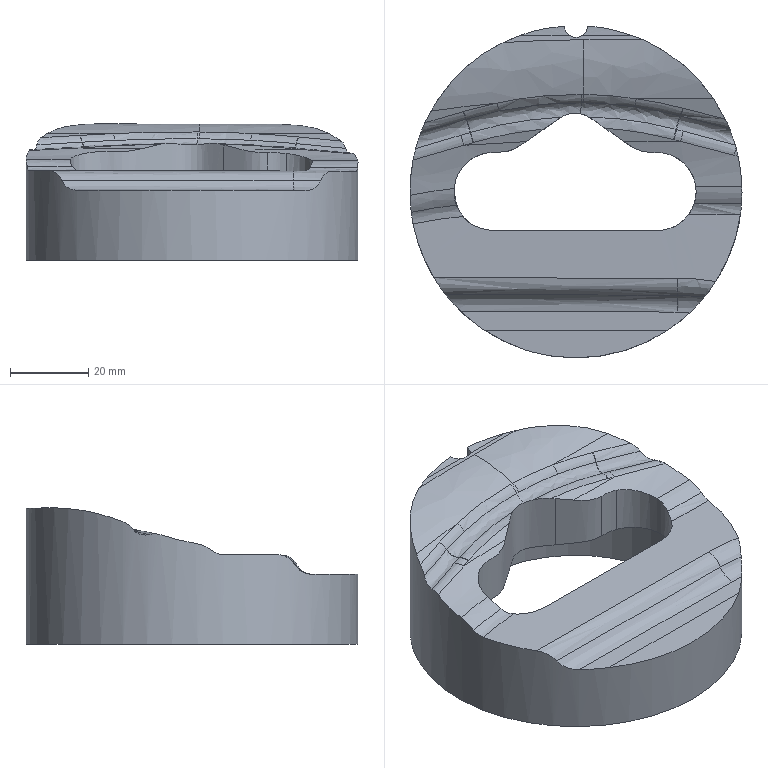Part | NX | features solid 2 | 1 solid | 54 faces | box 85 x 84.894 x 34.918 mm | volume 80240 mm3 | spline 49 | cylinder 3 | plane 2 | commonest cylinder face diameters 6 x1 67 x1 85 x1